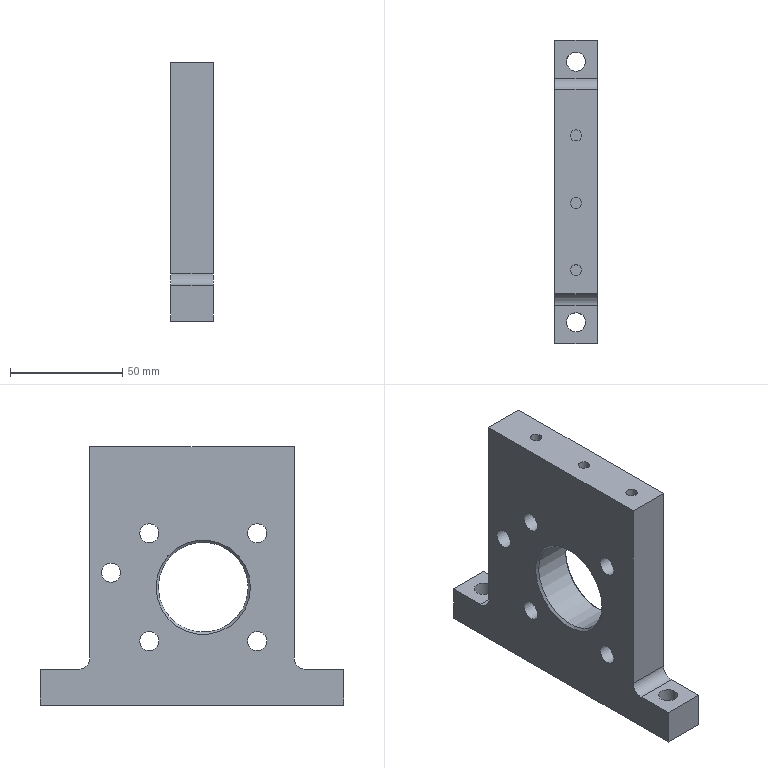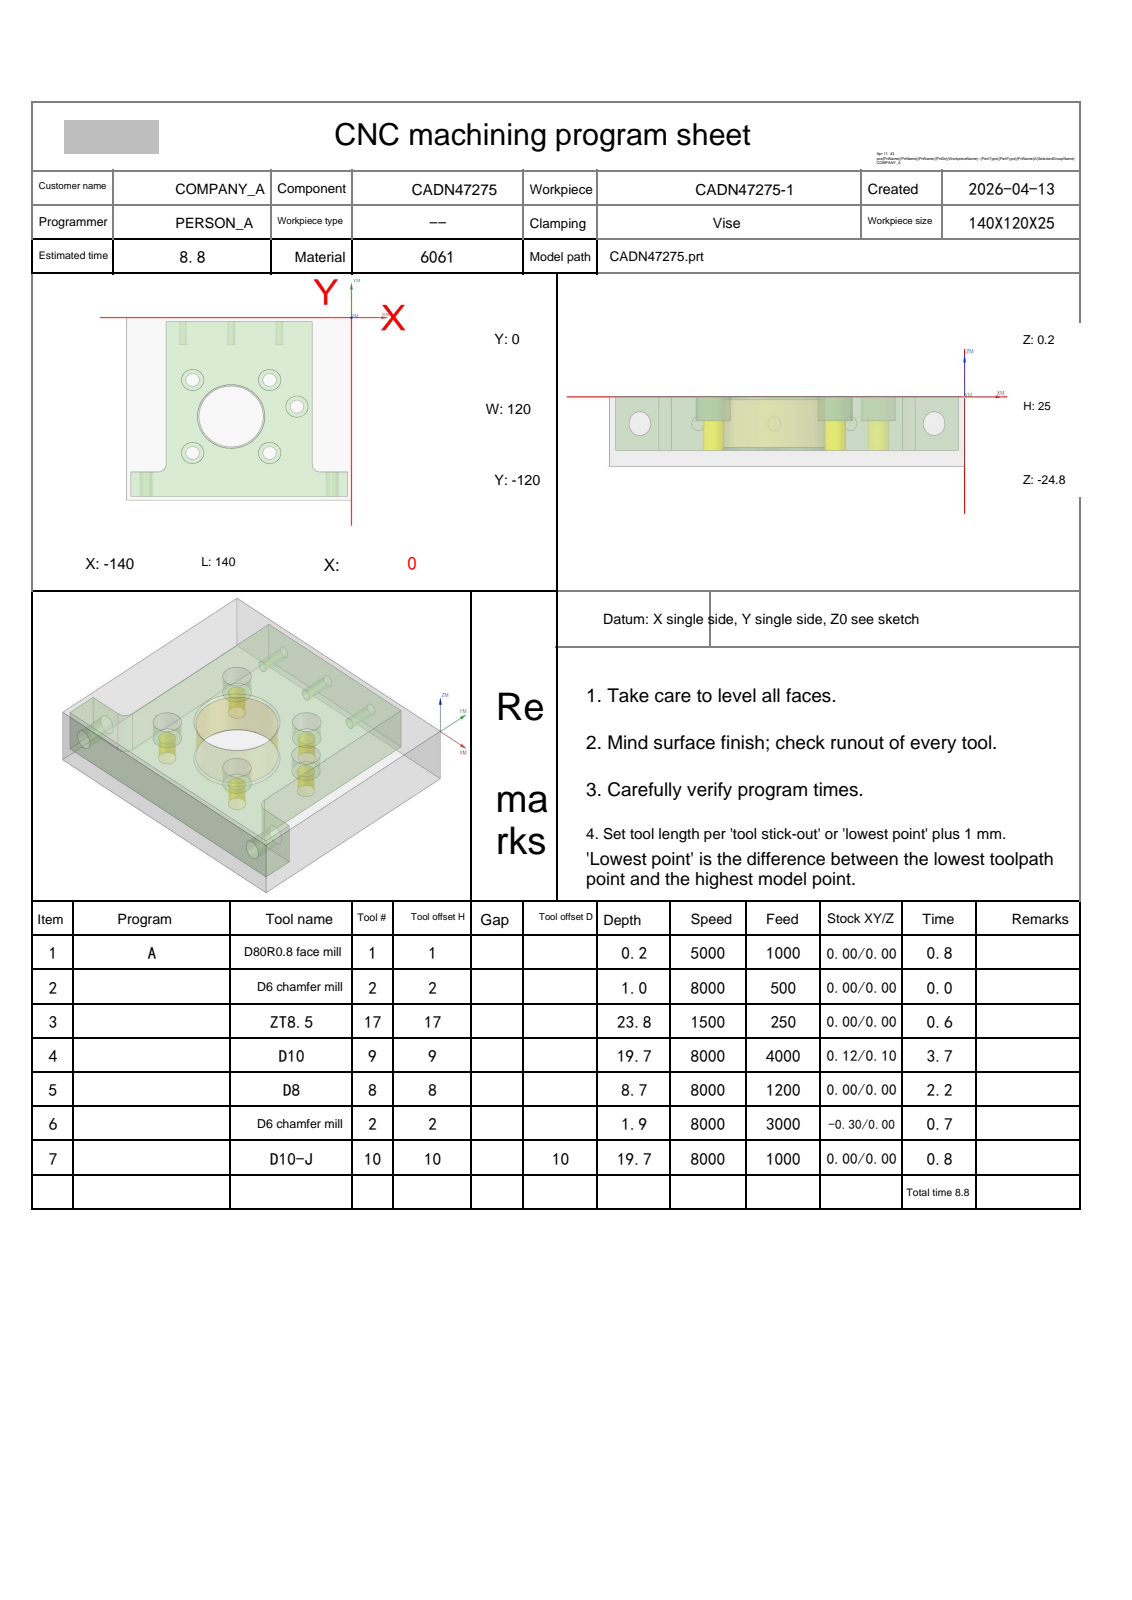NC program | NX | posted by the shop | part box 19 x 135 x 115 mm
Lines 1874 to 2456 of 2456:
N5 T08 M06
(D8  D=8. R=0. H=08 ce=0.10 di=0.00)
G00 G90 G54 X-34. Y-58.5 M03 S8000
G43 H08 Z20.
M08
Z.5
G03 X-32.55 Y-59.95 I1.45 J0.0 F1200.
X-31.1 Y-58.5 I0.0 J1.45
X-31.1 Y-58.5 Z0.0 I-2.9 J0.0
X-31.1 Y-58.5 Z-.5 I-2.9 J0.0
X-31.1 Y-58.5 Z-1. I-2.9 J0.0
X-31.1 Y-58.5 Z-1.5 I-2.9 J0.0
X-31.1 Y-58.5 Z-2. I-2.9 J0.0
X-31.1 Y-58.5 Z-2.5 I-2.9 J0.0
X-31.1 Y-58.5 Z-3. I-2.9 J0.0
X-31.1 Y-58.5 Z-3.5 I-2.9 J0.0
X-31.1 Y-58.5 Z-4. I-2.9 J0.0
X-31.1 Y-58.5 Z-4.5 I-2.9 J0.0
X-31.1 Y-58.5 Z-5. I-2.9 J0.0
X-31.1 Y-58.5 Z-5.5 I-2.9 J0.0
X-31.1 Y-58.5 Z-6. I-2.9 J0.0
X-31.1 Y-58.5 Z-6.5 I-2.9 J0.0
X-31.1 Y-58.5 Z-7. I-2.9 J0.0
X-31.1 Y-58.5 Z-7.5 I-2.9 J0.0
X-31.1 Y-58.5 Z-8. I-2.9 J0.0
X-31.1 Y-58.5 Z-8.5 I-2.9 J0.0
X-34. Y-55.6 I-2.9 J0.0
X-36.9 Y-58.5 I0.0 J-2.9
X-34. Y-61.4 I2.9 J0.0
X-31.1 Y-58.5 I0.0 J2.9
X-32.55 Y-57.05 I-1.45 J0.0
X-34. Y-58.5 I0.0 J-1.45
G00 Z20.
X-51. Y-41.
Z.5
G03 X-49.55 Y-42.45 I1.45 J0.0
X-48.1 Y-41. I0.0 J1.45
X-48.1 Y-41. Z0.0 I-2.9 J0.0
X-48.1 Y-41. Z-.5 I-2.9 J0.0
X-48.1 Y-41. Z-1. I-2.9 J0.0
X-48.1 Y-41. Z-1.5 I-2.9 J0.0
X-48.1 Y-41. Z-2. I-2.9 J0.0
X-48.1 Y-41. Z-2.5 I-2.9 J0.0
X-48.1 Y-41. Z-3. I-2.9 J0.0
X-48.1 Y-41. Z-3.5 I-2.9 J0.0
X-48.1 Y-41. Z-4. I-2.9 J0.0
X-48.1 Y-41. Z-4.5 I-2.9 J0.0
X-48.1 Y-41. Z-5. I-2.9 J0.0
X-48.1 Y-41. Z-5.5 I-2.9 J0.0
X-48.1 Y-41. Z-6. I-2.9 J0.0
X-48.1 Y-41. Z-6.5 I-2.9 J0.0
X-48.1 Y-41. Z-7. I-2.9 J0.0
X-48.1 Y-41. Z-7.5 I-2.9 J0.0
X-48.1 Y-41. Z-8. I-2.9 J0.0
X-48.1 Y-41. Z-8.5 I-2.9 J0.0
X-51. Y-38.1 I-2.9 J0.0
X-53.9 Y-41. I0.0 J-2.9
X-51. Y-43.9 I2.9 J0.0
X-48.1 Y-41. I0.0 J2.9
X-49.55 Y-39.55 I-1.45 J0.0
X-51. Y-41. I0.0 J-1.45
G00 Z20.
X-99.
Z.5
G03 X-97.55 Y-42.45 I1.45 J0.0
X-96.1 Y-41. I0.0 J1.45
X-96.1 Y-41. Z0.0 I-2.9 J0.0
X-96.1 Y-41. Z-.5 I-2.9 J0.0
X-96.1 Y-41. Z-1. I-2.9 J0.0
X-96.1 Y-41. Z-1.5 I-2.9 J0.0
X-96.1 Y-41. Z-2. I-2.9 J0.0
X-96.1 Y-41. Z-2.5 I-2.9 J0.0
X-96.1 Y-41. Z-3. I-2.9 J0.0
X-96.1 Y-41. Z-3.5 I-2.9 J0.0
X-96.1 Y-41. Z-4. I-2.9 J0.0
X-96.1 Y-41. Z-4.5 I-2.9 J0.0
X-96.1 Y-41. Z-5. I-2.9 J0.0
X-96.1 Y-41. Z-5.5 I-2.9 J0.0
X-96.1 Y-41. Z-6. I-2.9 J0.0
X-96.1 Y-41. Z-6.5 I-2.9 J0.0
X-96.1 Y-41. Z-7. I-2.9 J0.0
X-96.1 Y-41. Z-7.5 I-2.9 J0.0
X-96.1 Y-41. Z-8. I-2.9 J0.0
X-96.1 Y-41. Z-8.5 I-2.9 J0.0
X-99. Y-38.1 I-2.9 J0.0
X-101.9 Y-41. I0.0 J-2.9
X-99. Y-43.9 I2.9 J0.0
X-96.1 Y-41. I0.0 J2.9
X-97.55 Y-39.55 I-1.45 J0.0
X-99. Y-41. I0.0 J-1.45
G00 Z20.
Y-89.
Z.5
G03 X-97.55 Y-90.45 I1.45 J0.0
X-96.1 Y-89. I0.0 J1.45
X-96.1 Y-89. Z0.0 I-2.9 J0.0
X-96.1 Y-89. Z-.5 I-2.9 J0.0
X-96.1 Y-89. Z-1. I-2.9 J0.0
X-96.1 Y-89. Z-1.5 I-2.9 J0.0
X-96.1 Y-89. Z-2. I-2.9 J0.0
X-96.1 Y-89. Z-2.5 I-2.9 J0.0
X-96.1 Y-89. Z-3. I-2.9 J0.0
X-96.1 Y-89. Z-3.5 I-2.9 J0.0
X-96.1 Y-89. Z-4. I-2.9 J0.0
X-96.1 Y-89. Z-4.5 I-2.9 J0.0
X-96.1 Y-89. Z-5. I-2.9 J0.0
X-96.1 Y-89. Z-5.5 I-2.9 J0.0
X-96.1 Y-89. Z-6. I-2.9 J0.0
X-96.1 Y-89. Z-6.5 I-2.9 J0.0
X-96.1 Y-89. Z-7. I-2.9 J0.0
X-96.1 Y-89. Z-7.5 I-2.9 J0.0
X-96.1 Y-89. Z-8. I-2.9 J0.0
X-96.1 Y-89. Z-8.5 I-2.9 J0.0
X-99. Y-86.1 I-2.9 J0.0
X-101.9 Y-89. I0.0 J-2.9
X-99. Y-91.9 I2.9 J0.0
X-96.1 Y-89. I0.0 J2.9
X-97.55 Y-87.55 I-1.45 J0.0
X-99. Y-89. I0.0 J-1.45
G00 Z20.
X-51.
Z.5
G03 X-49.55 Y-90.45 I1.45 J0.0
X-48.1 Y-89. I0.0 J1.45
X-48.1 Y-89. Z0.0 I-2.9 J0.0
X-48.1 Y-89. Z-.5 I-2.9 J0.0
X-48.1 Y-89. Z-1. I-2.9 J0.0
X-48.1 Y-89. Z-1.5 I-2.9 J0.0
X-48.1 Y-89. Z-2. I-2.9 J0.0
X-48.1 Y-89. Z-2.5 I-2.9 J0.0
X-48.1 Y-89. Z-3. I-2.9 J0.0
X-48.1 Y-89. Z-3.5 I-2.9 J0.0
X-48.1 Y-89. Z-4. I-2.9 J0.0
X-48.1 Y-89. Z-4.5 I-2.9 J0.0
X-48.1 Y-89. Z-5. I-2.9 J0.0
X-48.1 Y-89. Z-5.5 I-2.9 J0.0
X-48.1 Y-89. Z-6. I-2.9 J0.0
X-48.1 Y-89. Z-6.5 I-2.9 J0.0
X-48.1 Y-89. Z-7. I-2.9 J0.0
X-48.1 Y-89. Z-7.5 I-2.9 J0.0
X-48.1 Y-89. Z-8. I-2.9 J0.0
X-48.1 Y-89. Z-8.5 I-2.9 J0.0
X-51. Y-86.1 I-2.9 J0.0
X-53.9 Y-89. I0.0 J-2.9
X-51. Y-91.9 I2.9 J0.0
X-48.1 Y-89. I0.0 J2.9
X-49.55 Y-87.55 I-1.45 J0.0
X-51. Y-89. I0.0 J-1.45
G00 Z20.
G00 G90 X-34. Y-58.5 M03 S8000
Z20.
Z.5
G41 D08
G01 X-33.973 Y-58.698 F500.
G03 X-32.493 Y-59.993 I1.48 J.198
X-31. Y-58.5 I0.0 J1.493
X-31. Y-58.5 Z-4.5 I-3. J0.0
X-33.073 Y-61.353 Z-8.5 I-3. J0.0
X-31. Y-58.5 I-.927 J2.853
X-34. Y-55.5 I-3. J0.0
X-37. Y-58.5 I0.0 J-3.
X-34. Y-61.5 I3. J0.0
X-33.073 Y-61.353 I0.0 J3.
X-32.041 Y-59.933 I-.461 J1.42
X-33.534 Y-58.44 I-1.493 J0.0
X-33.803 Y-58.464 I0.0 J-1.493
G01 G40 X-34. Y-58.5
G00 Z20.
X-51. Y-41.
Z.5
G41 D08
G01 X-50.973 Y-41.198
G03 X-49.493 Y-42.493 I1.48 J.198
X-48. Y-41. I0.0 J1.493
X-48. Y-41. Z-4.5 I-3. J0.0
X-50.073 Y-43.853 Z-8.5 I-3. J0.0
X-48. Y-41. I-.927 J2.853
X-51. Y-38. I-3. J0.0
X-54. Y-41. I0.0 J-3.
X-51. Y-44. I3. J0.0
X-50.073 Y-43.853 I0.0 J3.
X-49.041 Y-42.433 I-.461 J1.42
X-50.534 Y-40.94 I-1.493 J0.0
X-50.803 Y-40.964 I0.0 J-1.493
G01 G40 X-51. Y-41.
G00 Z20.
X-99.
Z.5
G41 D08
G01 X-98.973 Y-41.198
G03 X-97.493 Y-42.493 I1.48 J.198
X-96. Y-41. I0.0 J1.493
X-96. Y-41. Z-4.5 I-3. J0.0
X-98.073 Y-43.853 Z-8.5 I-3. J0.0
X-96. Y-41. I-.927 J2.853
X-99. Y-38. I-3. J0.0
X-102. Y-41. I0.0 J-3.
X-99. Y-44. I3. J0.0
X-98.073 Y-43.853 I0.0 J3.
X-97.041 Y-42.433 I-.461 J1.42
X-98.534 Y-40.94 I-1.493 J0.0
X-98.803 Y-40.964 I0.0 J-1.493
G01 G40 X-99. Y-41.
G00 Z20.
Y-89.
Z.5
G41 D08
G01 X-98.973 Y-89.198
G03 X-97.493 Y-90.493 I1.48 J.198
X-96. Y-89. I0.0 J1.493
X-96. Y-89. Z-4.5 I-3. J0.0
X-98.073 Y-91.853 Z-8.5 I-3. J0.0
X-96. Y-89. I-.927 J2.853
X-99. Y-86. I-3. J0.0
X-102. Y-89. I0.0 J-3.
X-99. Y-92. I3. J0.0
X-98.073 Y-91.853 I0.0 J3.
X-97.041 Y-90.433 I-.461 J1.42
X-98.534 Y-88.94 I-1.493 J0.0
X-98.803 Y-88.964 I0.0 J-1.493
G01 G40 X-99. Y-89.
G00 Z20.
X-51.
Z.5
G41 D08
G01 X-50.973 Y-89.198
G03 X-49.493 Y-90.493 I1.48 J.198
X-48. Y-89. I0.0 J1.493
X-48. Y-89. Z-4.5 I-3. J0.0
X-50.073 Y-91.853 Z-8.5 I-3. J0.0
X-48. Y-89. I-.927 J2.853
X-51. Y-86. I-3. J0.0
X-54. Y-89. I0.0 J-3.
X-51. Y-92. I3. J0.0
X-50.073 Y-91.853 I0.0 J3.
X-49.041 Y-90.433 I-.461 J1.42
X-50.534 Y-88.94 I-1.493 J0.0
X-50.803 Y-88.964 I0.0 J-1.493
G01 G40 X-51. Y-89.
G00 Z20.
G91 G28 Z0.0
M05
M09
G91 G28 Z0.0
M01
N6 T02 M06
(D6 chamfer mill  D=6. R=0. H=02 ce=0.00 di=0.00)
G00 G90 G54 X-69.75 Y-119.628 M03 S8000
G43 H02 Z20.
M08
Z2.099
G01 Z-1.5 F3000.
G03 X-69.67 Y-119.328 I-.52 J.3
X-69.97 Y-118.808 I-.6 J0.0
G01 X-70. Y-118.8
X-137.5
G02 X-138.8 Y-117.5 I0.0 J1.3
G01 Y-101.5
G02 X-137.5 Y-100.2 I1.3 J0.0
G01 X-120.5
G03 X-116.8 Y-96.5 I0.0 J3.7
G01 Y-2.5
G02 X-115.5 Y-1.2 I1.3 J0.0
G01 X-24.5
G02 X-23.2 Y-2.5 I0.0 J-1.3
G01 Y-96.5
G03 X-19.5 Y-100.2 I3.7 J0.0
G01 X-2.5
G02 X-1.2 Y-101.5 I0.0 J-1.3
G01 Y-117.5
G02 X-2.5 Y-118.8 I-1.3 J0.0
G01 X-70.
X-70.03 Y-118.808
G03 X-70.33 Y-119.328 I.3 J-.52
X-70.25 Y-119.628 I.6 J0.0
G01 Z2.099
G00 Z20.
X-50.703 Y-84.112
Z2.133
G01 Z-1.5
G03 X-50.639 Y-83.842 I-.536 J.269
X-50.97 Y-83.306 I-.6 J0.0
G01 X-51. Y-83.3
G03 X-56.7 Y-89. I0.0 J-5.7
X-51. Y-94.7 I5.7 J0.0
X-45.3 Y-89. I0.0 J5.7
X-51. Y-83.3 I-5.7 J0.0
G01 X-51.03 Y-83.306
G03 X-51.361 Y-83.842 I.269 J-.536
X-51.297 Y-84.112 I.6 J0.0
G01 Z2.131
G00 Z20.
X-34.297 Y-63.388
Z2.133
G01 Z-1.5
G03 X-34.361 Y-63.658 I.536 J-.269
X-34.03 Y-64.194 I.6 J0.0
G01 X-34. Y-64.2
G03 X-28.3 Y-58.5 I0.0 J5.7
X-34. Y-52.8 I-5.7 J0.0
X-39.7 Y-58.5 I0.0 J-5.7
X-34. Y-64.2 I5.7 J0.0
G01 X-33.97 Y-64.194
G03 X-33.639 Y-63.658 I-.269 J.536
X-33.703 Y-63.388 I-.6 J0.0
G01 Z2.131
G00 Z20.
X-50.703 Y-36.112
Z2.133
G01 Z-1.5
G03 X-50.639 Y-35.842 I-.536 J.269
X-50.97 Y-35.306 I-.6 J0.0
G01 X-51. Y-35.3
G03 X-56.7 Y-41. I0.0 J-5.7
X-51. Y-46.7 I5.7 J0.0
X-45.3 Y-41. I0.0 J5.7
X-51. Y-35.3 I-5.7 J0.0
G01 X-51.03 Y-35.306
G03 X-51.361 Y-35.842 I.269 J-.536
X-51.297 Y-36.112 I.6 J0.0
G01 Z2.131
G00 Z20.
X-98.703
Z2.133
G01 Z-1.5
G03 X-98.639 Y-35.842 I-.536 J.269
X-98.97 Y-35.306 I-.6 J0.0
G01 X-99. Y-35.3
G03 X-104.7 Y-41. I0.0 J-5.7
X-99. Y-46.7 I5.7 J0.0
X-93.3 Y-41. I0.0 J5.7
X-99. Y-35.3 I-5.7 J0.0
G01 X-99.03 Y-35.306
G03 X-99.361 Y-35.842 I.269 J-.536
X-99.297 Y-36.112 I.6 J0.0
G01 Z2.131
G00 Z20.
X-98.703 Y-84.112
Z2.133
G01 Z-1.5
G03 X-98.639 Y-83.842 I-.536 J.269
X-98.97 Y-83.306 I-.6 J0.0
G01 X-99. Y-83.3
G03 X-104.7 Y-89. I0.0 J-5.7
X-99. Y-94.7 I5.7 J0.0
X-93.3 Y-89. I0.0 J5.7
X-99. Y-83.3 I-5.7 J0.0
G01 X-99.03 Y-83.306
G03 X-99.361 Y-83.842 I.269 J-.536
X-99.297 Y-84.112 I.6 J0.0
G01 Z2.131
G00 Z20.
G00 G90 X-105.292 Y-41.281 M03 S8000
Z20.
Z2.5
G01 X-105.271 Y-41.63 Z2.373 F800.
X-105.196 Y-42.158 Z2.179
X-105.075 Y-42.678 Z1.984
X-104.912 Y-43.186 Z1.79
X-104.706 Y-43.678 Z1.596
X-104.459 Y-44.152 Z1.402
X-104.172 Y-44.602 Z1.207
X-103.849 Y-45.027 Z1.013
X-103.491 Y-45.422 Z.819
X-103.101 Y-45.786 Z.625
X-102.681 Y-46.116 Z.43
X-102.235 Y-46.409 Z.236
X-101.766 Y-46.664 Z.042
X-101.277 Y-46.877 Z-.152
X-100.772 Y-47.049 Z-.347
X-100.254 Y-47.177 Z-.541
X-99.727 Y-47.261 Z-.735
X-99.194 Y-47.3 Z-.929
X-99. Z-1.
G03 X-92.7 Y-41. I0.0 J6.3
X-99. Y-34.7 I-6.3 J0.0
X-105.3 Y-41. I0.0 J-6.3
X-99. Y-47.3 I6.3 J0.0
X-98.501 Y-47.28 I0.0 J6.3
G01 Z1.5
G00 Z20.
X-57.292 Y-41.281
Z2.5
G01 X-57.271 Y-41.63 Z2.373
X-57.196 Y-42.158 Z2.179
X-57.075 Y-42.678 Z1.984
X-56.912 Y-43.186 Z1.79
X-56.706 Y-43.678 Z1.596
X-56.459 Y-44.152 Z1.402
X-56.172 Y-44.602 Z1.207
X-55.849 Y-45.027 Z1.013
X-55.491 Y-45.422 Z.819
X-55.101 Y-45.786 Z.625
X-54.681 Y-46.116 Z.43
X-54.235 Y-46.409 Z.236
X-53.766 Y-46.664 Z.042
X-53.277 Y-46.877 Z-.152
X-52.772 Y-47.049 Z-.347
X-52.254 Y-47.177 Z-.541
X-51.727 Y-47.261 Z-.735
X-51.194 Y-47.3 Z-.929
X-51. Z-1.
G03 X-44.7 Y-41. I0.0 J6.3
X-51. Y-34.7 I-6.3 J0.0
X-57.3 Y-41. I0.0 J-6.3
X-51. Y-47.3 I6.3 J0.0
X-50.501 Y-47.28 I0.0 J6.3
G01 Z1.5
G00 Z20.
X-27.708 Y-58.219
Z2.5
G01 X-27.729 Y-57.87 Z2.373
X-27.804 Y-57.342 Z2.179
X-27.925 Y-56.822 Z1.984
X-28.088 Y-56.314 Z1.79
X-28.294 Y-55.822 Z1.596
X-28.541 Y-55.349 Z1.402
X-28.828 Y-54.898 Z1.207
X-29.151 Y-54.473 Z1.013
X-29.509 Y-54.078 Z.819
X-29.899 Y-53.714 Z.625
X-30.319 Y-53.384 Z.43
X-30.765 Y-53.091 Z.236
X-31.234 Y-52.836 Z.042
X-31.723 Y-52.623 Z-.152
X-32.228 Y-52.451 Z-.347
X-32.746 Y-52.323 Z-.541
X-33.273 Y-52.239 Z-.735
X-33.806 Y-52.2 Z-.929
X-34. Z-1.
G03 X-40.3 Y-58.5 I0.0 J-6.3
X-34. Y-64.8 I6.3 J0.0
X-27.7 Y-58.5 I0.0 J6.3
X-34. Y-52.2 I-6.3 J0.0
X-34.499 Y-52.22 I0.0 J-6.3
G01 Z1.5
G00 Z20.
X-57.292 Y-89.281
Z2.5
G01 X-57.271 Y-89.63 Z2.373
X-57.196 Y-90.158 Z2.179
X-57.075 Y-90.678 Z1.984
X-56.912 Y-91.186 Z1.79
X-56.706 Y-91.678 Z1.596
X-56.459 Y-92.152 Z1.402
X-56.172 Y-92.602 Z1.207
X-55.849 Y-93.027 Z1.013
X-55.491 Y-93.422 Z.819
X-55.101 Y-93.786 Z.625
X-54.681 Y-94.116 Z.43
X-54.235 Y-94.409 Z.236
X-53.766 Y-94.664 Z.042
X-53.277 Y-94.877 Z-.152
X-52.772 Y-95.049 Z-.347
X-52.254 Y-95.177 Z-.541
X-51.727 Y-95.261 Z-.735
X-51.194 Y-95.3 Z-.929
X-51. Z-1.
G03 X-44.7 Y-89. I0.0 J6.3
X-51. Y-82.7 I-6.3 J0.0
X-57.3 Y-89. I0.0 J-6.3
X-51. Y-95.3 I6.3 J0.0
X-50.501 Y-95.28 I0.0 J6.3
G01 Z1.5
G00 Z20.
X-105.292 Y-89.281
Z2.5
G01 X-105.271 Y-89.63 Z2.373
X-105.196 Y-90.158 Z2.179
X-105.075 Y-90.678 Z1.984
X-104.912 Y-91.186 Z1.79
X-104.706 Y-91.678 Z1.596
X-104.459 Y-92.152 Z1.402
X-104.172 Y-92.602 Z1.207
X-103.849 Y-93.027 Z1.013
X-103.491 Y-93.422 Z.819
X-103.101 Y-93.786 Z.625
X-102.681 Y-94.116 Z.43
X-102.235 Y-94.409 Z.236
X-101.766 Y-94.664 Z.042
X-101.277 Y-94.877 Z-.152
X-100.772 Y-95.049 Z-.347
X-100.254 Y-95.177 Z-.541
X-99.727 Y-95.261 Z-.735
X-99.194 Y-95.3 Z-.929
X-99. Z-1.
G03 X-92.7 Y-89. I0.0 J6.3
X-99. Y-82.7 I-6.3 J0.0
X-105.3 Y-89. I0.0 J-6.3
X-99. Y-95.3 I6.3 J0.0
X-98.501 Y-95.28 I0.0 J6.3
G01 Z1.5
G00 Z20.
G00 G90 X-76.2 Y-83.06 M03 S6500
Z20.
Z-.2
G01 Z-1.7 F1500.
Y-83.1
G03 X-75. Y-84.3 I1.2 J0.0
X-55.7 Y-65. I0.0 J19.3
X-75. Y-45.7 I-19.3 J0.0
X-94.3 Y-65. I0.0 J-19.3
X-75. Y-84.3 I19.3 J0.0
X-74.6 Y-84.296 I0.0 J19.3
X-73.425 Y-83.096 I-.025 J1.2
G01 Y-83.071
X-73.426 Y-83.031
Z-.2
G00 Z20.
G91 G28 Z0.0
M05
M09
G91 G28 Z0.0
M01
N7 T10 M06
(D10-J  D=10. R=0. H=10 ce=0.00 di=0.00)
G00 G90 G54 X-76.5 Y-78.216 M03 S8000
G43 H10 Z10.2
M08
Z-8.5
G01 Z-10. F1000.
G41 D10
Y-78.5
G03 X-75. Y-80. I1.5 J0.0
X-60. Y-65. I0.0 J15.
X-75. Y-50. I-15. J0.0
X-90. Y-65. I0.0 J-15.
X-75. Y-80. I15. J0.0
X-74.6 Y-79.995 I0.0 J15.
X-73.14 Y-78.495 I-.04 J1.499
G01 X-73.141 Y-78.455
X-73.143 Y-78.372
G40 X-73.148 Y-78.172
Z-8.5
G00 X-76.5 Y-78.216
Z-17.5
G01 Z-19.
G41 D10
Y-78.5
G03 X-75. Y-80. I1.5 J0.0
X-60. Y-65. I0.0 J15.
X-75. Y-50. I-15. J0.0
X-90. Y-65. I0.0 J-15.
X-75. Y-80. I15. J0.0
X-74.6 Y-79.995 I0.0 J15.
X-73.14 Y-78.495 I-.04 J1.499
G01 X-73.141 Y-78.455
X-73.143 Y-78.372
G40 X-73.148 Y-78.172
Z-17.5
G00 Z10.2
G00 G90 X-1.487 Y-123.616 M03 S8000
Z20.
Z-19.
G01 Z-19.5 F1000.
G41 D10
X-1.503 Y-123.417
G03 X-2.5 Y-122.5 I-.997 J-.083
G01 X-137.5
G02 X-142.5 Y-117.5 I0.0 J5.
G01 Y-101.5
G02 X-137.5 Y-96.5 I5. J0.0
G01 X-120.5
Y-2.5
G02 X-115.5 Y2.5 I5. J0.0
G01 X-24.5
G02 X-19.5 Y-2.5 I0.0 J-5.
G01 Y-96.5
X-2.5
G02 X2.5 Y-101.5 I0.0 J-5.
G01 Y-117.5
G02 X-2.5 Y-122.5 I-5. J0.0
G01 X-3.
G03 X-4. Y-123.5 I0.0 J-1.
G01 G40 Y-123.7
Z-19.
G00 Z20.
M05
M09
G91 G28 Z0.0
G91 G28 Y0.0
M30
%